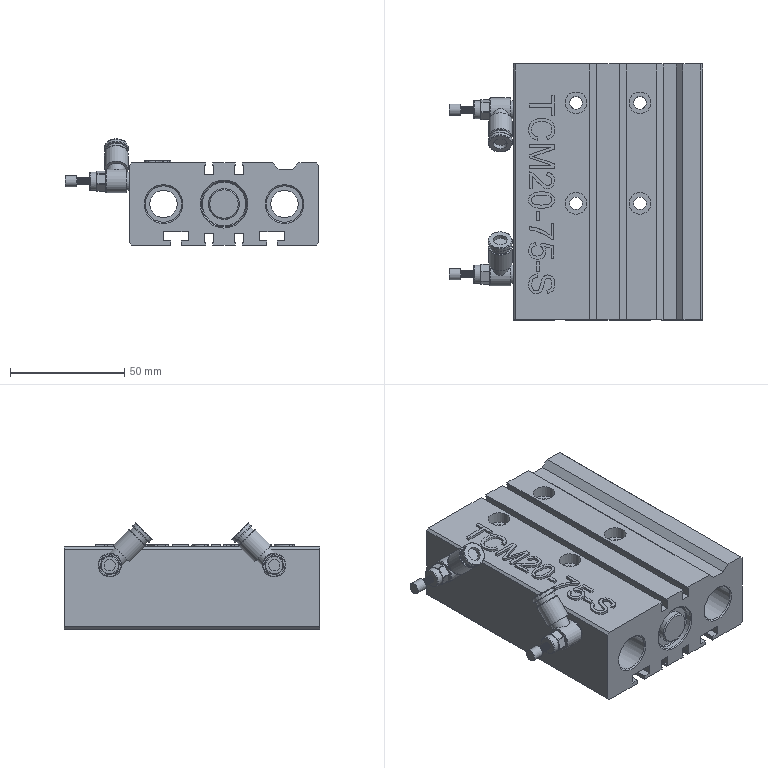Part | STEP file | Tube necking machine_id726_x_t | 1 solid | 379 faces | box 111 x 112 x 46.543 mm | volume 281907 mm3 | plane 254 | other 62 | cylinder 37 | torus 12 | spline 8 | cone 6 | commonest cylinder face diameters 8 x6 5.5 x4 9.5 x4 10.3 x4 2.5 x2 3 x2